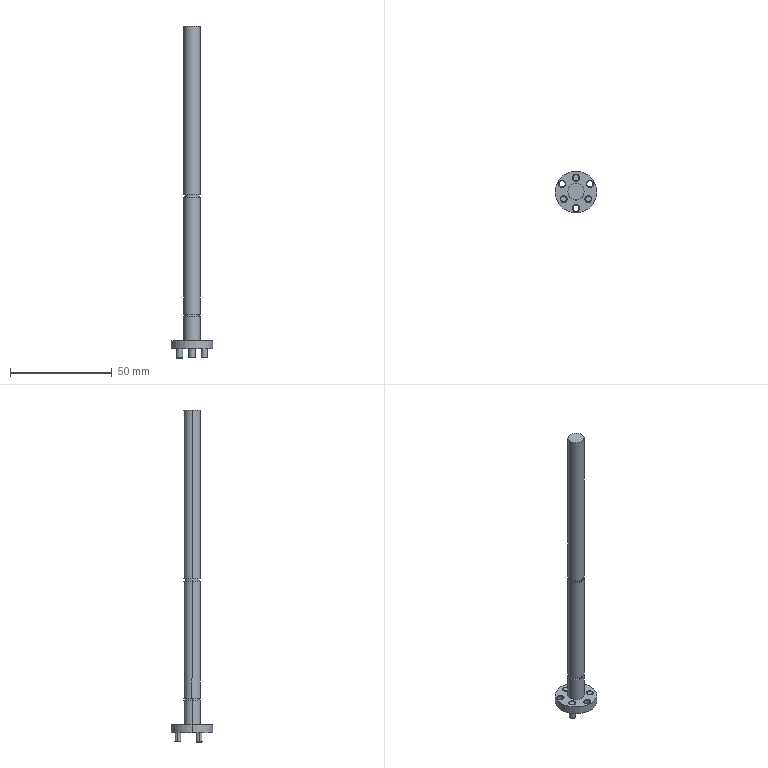Part | SolidWorks | features ICE 2, BaseBody 1 | 1 solid | 88 faces | box 20.5 x 20.5 x 163.5 mm | volume 9096 mm3 | cylinder 30 | cone 28 | plane 18 | torus 12 | commonest cylinder face diameters 3 x18 8 x6 7.2 x4 20.5 x2